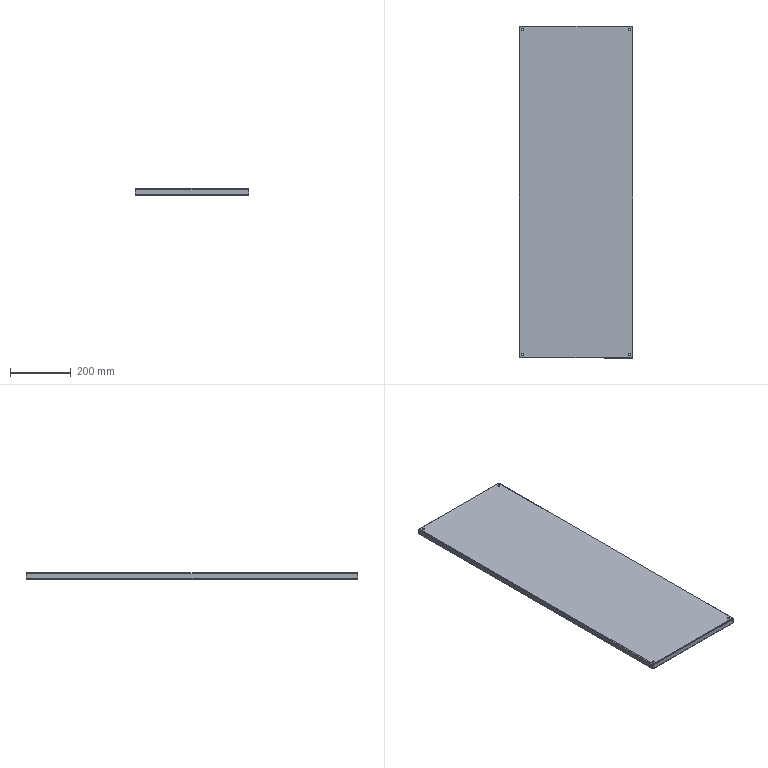Part | SolidWorks | features EdgeFlange 2, FlatPattern 1, HoleWzd 1, SMBaseFlange 1, SheetMetal 1 | 1 solid | 98 faces | box 376 x 1096 x 20 mm | volume 1022665 mm3 | plane 46 | cylinder 36 | spline 16 | commonest cylinder face diameters 7 x20 1.473 x8 5.473 x8